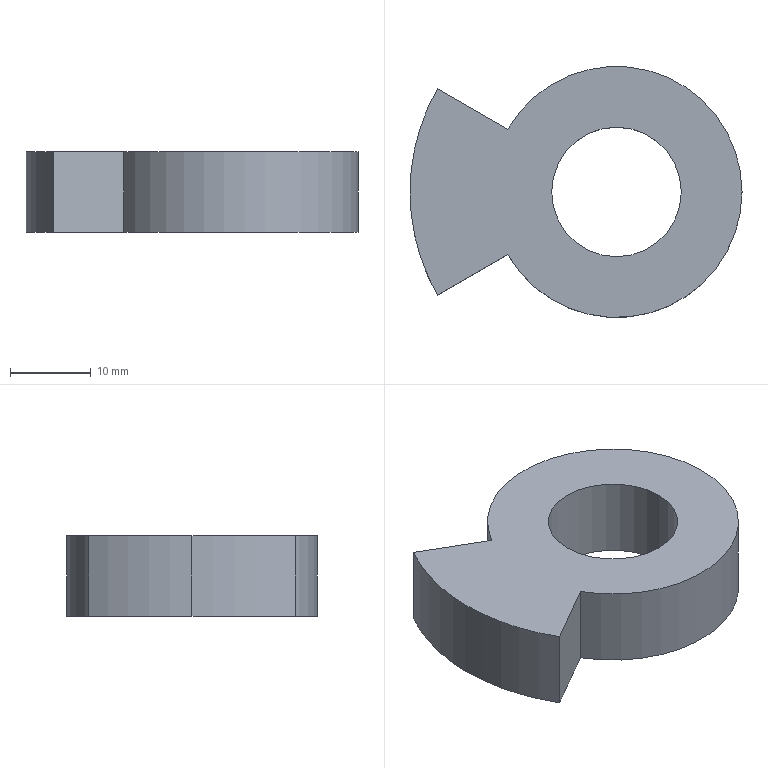Part | STEP file | Sensing plate | 1 solid | 9 faces | box 41 x 31 x 10 mm | volume 7684 mm3 | cylinder 5 | plane 4 | commonest cylinder face diameters 16 x2 51 x2 31 x1
STEP:
#1=CARTESIAN_POINT('',(-8.,0.,5.));
#2=VERTEX_POINT('',#1);
#3=CARTESIAN_POINT('',(8.,0.,5.));
#4=VERTEX_POINT('',#3);
#5=CARTESIAN_POINT('',(0.,0.,5.));
#6=DIRECTION('',(0.,0.,1.));
#7=DIRECTION('',(1.,0.,0.));
#8=AXIS2_PLACEMENT_3D('',#5,#6,#7);
#9=CIRCLE('',#8,8.);
#10=EDGE_CURVE('',#2,#4,#9,.T.);
#11=ORIENTED_EDGE('',*,*,#10,.T.);
#12=CARTESIAN_POINT('',(8.,0.,-5.));
#13=VERTEX_POINT('',#12);
#14=CARTESIAN_POINT('',(8.,0.,5.));
#15=DIRECTION('',(0.,0.,-1.));
#16=VECTOR('',#15,1000.);
#17=LINE('',#14,#16);
#18=EDGE_CURVE('',#4,#13,#17,.T.);
#19=ORIENTED_EDGE('',*,*,#18,.T.);
#20=CARTESIAN_POINT('',(-8.,0.,-5.));
#21=VERTEX_POINT('',#20);
#22=CARTESIAN_POINT('',(0.,0.,-5.));
#23=DIRECTION('',(0.,0.,1.));
#24=DIRECTION('',(1.,0.,0.));
#25=AXIS2_PLACEMENT_3D('',#22,#23,#24);
#26=CIRCLE('',#25,8.);
#27=EDGE_CURVE('',#21,#13,#26,.T.);
#28=ORIENTED_EDGE('',*,*,#27,.F.);
#29=CARTESIAN_POINT('',(-8.,0.,5.));
#30=DIRECTION('',(0.,0.,-1.));
#31=VECTOR('',#30,1000.);
#32=LINE('',#29,#31);
#33=EDGE_CURVE('',#2,#21,#32,.T.);
#34=ORIENTED_EDGE('',*,*,#33,.F.);
#35=EDGE_LOOP('',(#11,#19,#28,#34));
#36=FACE_OUTER_BOUND('',#35,.T.);
#37=CARTESIAN_POINT('',(0.,0.,5.));
#38=DIRECTION('',(0.,0.,-1.));
#39=DIRECTION('',(-1.,0.,0.));
#40=AXIS2_PLACEMENT_3D('',#37,#38,#39);
#41=CYLINDRICAL_SURFACE('',#40,8.);
#42=ADVANCED_FACE('',(#36),#41,.F.);
#43=CARTESIAN_POINT('',(-25.5,0.,5.));
#44=VERTEX_POINT('',#43);
#45=CARTESIAN_POINT('',(-22.084,-12.75,5.));
#46=VERTEX_POINT('',#45);
#47=CARTESIAN_POINT('',(0.,0.,5.));
#48=DIRECTION('',(0.,0.,1.));
#49=DIRECTION('',(1.,0.,0.));
#50=AXIS2_PLACEMENT_3D('',#47,#48,#49);
#51=CIRCLE('',#50,25.5);
#52=EDGE_CURVE('',#44,#46,#51,.T.);
#53=ORIENTED_EDGE('',*,*,#52,.F.);
#54=CARTESIAN_POINT('',(-25.5,0.,-5.));
#55=VERTEX_POINT('',#54);
#56=CARTESIAN_POINT('',(-25.5,0.,5.));
#57=DIRECTION('',(0.,0.,-1.));
#58=VECTOR('',#57,1000.);
#59=LINE('',#56,#58);
#60=EDGE_CURVE('',#44,#55,#59,.T.);
#61=ORIENTED_EDGE('',*,*,#60,.T.);
#62=CARTESIAN_POINT('',(-22.084,-12.75,-5.));
#63=VERTEX_POINT('',#62);
#64=CARTESIAN_POINT('',(0.,0.,-5.));
#65=DIRECTION('',(0.,0.,1.));
#66=DIRECTION('',(1.,0.,0.));
#67=AXIS2_PLACEMENT_3D('',#64,#65,#66);
#68=CIRCLE('',#67,25.5);
#69=EDGE_CURVE('',#55,#63,#68,.T.);
#70=ORIENTED_EDGE('',*,*,#69,.T.);
#71=CARTESIAN_POINT('',(-22.084,-12.75,5.));
#72=DIRECTION('',(0.,0.,-1.));
#73=VECTOR('',#72,1000.);
#74=LINE('',#71,#73);
#75=EDGE_CURVE('',#46,#63,#74,.T.);
#76=ORIENTED_EDGE('',*,*,#75,.F.);
#77=EDGE_LOOP('',(#53,#61,#70,#76));
#78=FACE_OUTER_BOUND('',#77,.T.);
#79=CARTESIAN_POINT('',(0.,0.,5.));
#80=DIRECTION('',(0.,0.,-1.));
#81=DIRECTION('',(-1.,0.,0.));
#82=AXIS2_PLACEMENT_3D('',#79,#80,#81);
#83=CYLINDRICAL_SURFACE('',#82,25.5);
#84=ADVANCED_FACE('',(#78),#83,.T.);
#85=CARTESIAN_POINT('',(-13.423,-7.75,-5.));
#86=VERTEX_POINT('',#85);
#87=CARTESIAN_POINT('',(0.,0.,-5.));
#88=DIRECTION('',(-0.866,-0.5,0.));
#89=VECTOR('',#88,1000.);
#90=LINE('',#87,#89);
#91=EDGE_CURVE('',#86,#63,#90,.T.);
#92=ORIENTED_EDGE('',*,*,#91,.F.);
#93=CARTESIAN_POINT('',(-13.423,-7.75,5.));
#94=VERTEX_POINT('',#93);
#95=CARTESIAN_POINT('',(-13.423,-7.75,5.));
#96=DIRECTION('',(0.,0.,-1.));
#97=VECTOR('',#96,1000.);
#98=LINE('',#95,#97);
#99=EDGE_CURVE('',#94,#86,#98,.T.);
#100=ORIENTED_EDGE('',*,*,#99,.F.);
#101=CARTESIAN_POINT('',(0.,0.,5.));
#102=DIRECTION('',(-0.866,-0.5,0.));
#103=VECTOR('',#102,1000.);
#104=LINE('',#101,#103);
#105=EDGE_CURVE('',#94,#46,#104,.T.);
#106=ORIENTED_EDGE('',*,*,#105,.T.);
#107=ORIENTED_EDGE('',*,*,#75,.T.);
#108=EDGE_LOOP('',(#92,#100,#106,#107));
#109=FACE_OUTER_BOUND('',#108,.T.);
#110=CARTESIAN_POINT('',(0.,0.,5.));
#111=DIRECTION('',(0.5,-0.866,0.));
#112=DIRECTION('',(0.866,0.5,0.));
#113=AXIS2_PLACEMENT_3D('',#110,#111,#112);
#114=PLANE('',#113);
#115=ADVANCED_FACE('',(#109),#114,.T.);
#116=CARTESIAN_POINT('',(-13.423,7.75,-5.));
#117=VERTEX_POINT('',#116);
#118=CARTESIAN_POINT('',(0.,0.,-5.));
#119=DIRECTION('',(0.,0.,1.));
#120=DIRECTION('',(1.,0.,0.));
#121=AXIS2_PLACEMENT_3D('',#118,#119,#120);
#122=CIRCLE('',#121,15.5);
#123=EDGE_CURVE('',#86,#117,#122,.T.);
#124=ORIENTED_EDGE('',*,*,#123,.T.);
#125=CARTESIAN_POINT('',(-13.423,7.75,5.));
#126=VERTEX_POINT('',#125);
#127=CARTESIAN_POINT('',(-13.423,7.75,5.));
#128=DIRECTION('',(0.,0.,-1.));
#129=VECTOR('',#128,1000.);
#130=LINE('',#127,#129);
#131=EDGE_CURVE('',#126,#117,#130,.T.);
#132=ORIENTED_EDGE('',*,*,#131,.F.);
#133=CARTESIAN_POINT('',(0.,0.,5.));
#134=DIRECTION('',(0.,0.,1.));
#135=DIRECTION('',(1.,0.,0.));
#136=AXIS2_PLACEMENT_3D('',#133,#134,#135);
#137=CIRCLE('',#136,15.5);
#138=EDGE_CURVE('',#94,#126,#137,.T.);
#139=ORIENTED_EDGE('',*,*,#138,.F.);
#140=ORIENTED_EDGE('',*,*,#99,.T.);
#141=EDGE_LOOP('',(#124,#132,#139,#140));
#142=FACE_OUTER_BOUND('',#141,.T.);
#143=CARTESIAN_POINT('',(0.,0.,5.));
#144=DIRECTION('',(0.,0.,-1.));
#145=DIRECTION('',(-1.,0.,0.));
#146=AXIS2_PLACEMENT_3D('',#143,#144,#145);
#147=CYLINDRICAL_SURFACE('',#146,15.5);
#148=ADVANCED_FACE('',(#142),#147,.T.);
#149=CARTESIAN_POINT('',(-22.084,12.75,-5.));
#150=VERTEX_POINT('',#149);
#151=CARTESIAN_POINT('',(0.,0.,-5.));
#152=DIRECTION('',(-0.866,0.5,0.));
#153=VECTOR('',#152,1000.);
#154=LINE('',#151,#153);
#155=EDGE_CURVE('',#117,#150,#154,.T.);
#156=ORIENTED_EDGE('',*,*,#155,.T.);
#157=CARTESIAN_POINT('',(-22.084,12.75,5.));
#158=VERTEX_POINT('',#157);
#159=CARTESIAN_POINT('',(-22.084,12.75,5.));
#160=DIRECTION('',(0.,0.,-1.));
#161=VECTOR('',#160,1000.);
#162=LINE('',#159,#161);
#163=EDGE_CURVE('',#158,#150,#162,.T.);
#164=ORIENTED_EDGE('',*,*,#163,.F.);
#165=CARTESIAN_POINT('',(0.,0.,5.));
#166=DIRECTION('',(-0.866,0.5,0.));
#167=VECTOR('',#166,1000.);
#168=LINE('',#165,#167);
#169=EDGE_CURVE('',#126,#158,#168,.T.);
#170=ORIENTED_EDGE('',*,*,#169,.F.);
#171=ORIENTED_EDGE('',*,*,#131,.T.);
#172=EDGE_LOOP('',(#156,#164,#170,#171));
#173=FACE_OUTER_BOUND('',#172,.T.);
#174=CARTESIAN_POINT('',(0.,0.,5.));
#175=DIRECTION('',(-0.5,-0.866,0.));
#176=DIRECTION('',(0.866,-0.5,0.));
#177=AXIS2_PLACEMENT_3D('',#174,#175,#176);
#178=PLANE('',#177);
#179=ADVANCED_FACE('',(#173),#178,.F.);
#180=ORIENTED_EDGE('',*,*,#60,.F.);
#181=CARTESIAN_POINT('',(0.,0.,5.));
#182=DIRECTION('',(0.,0.,1.));
#183=DIRECTION('',(1.,0.,0.));
#184=AXIS2_PLACEMENT_3D('',#181,#182,#183);
#185=CIRCLE('',#184,25.5);
#186=EDGE_CURVE('',#158,#44,#185,.T.);
#187=ORIENTED_EDGE('',*,*,#186,.F.);
#188=ORIENTED_EDGE('',*,*,#163,.T.);
#189=CARTESIAN_POINT('',(0.,0.,-5.));
#190=DIRECTION('',(0.,0.,1.));
#191=DIRECTION('',(1.,0.,0.));
#192=AXIS2_PLACEMENT_3D('',#189,#190,#191);
#193=CIRCLE('',#192,25.5);
#194=EDGE_CURVE('',#150,#55,#193,.T.);
#195=ORIENTED_EDGE('',*,*,#194,.T.);
#196=EDGE_LOOP('',(#180,#187,#188,#195));
#197=FACE_OUTER_BOUND('',#196,.T.);
#198=CARTESIAN_POINT('',(0.,0.,5.));
#199=DIRECTION('',(0.,0.,-1.));
#200=DIRECTION('',(-1.,0.,0.));
#201=AXIS2_PLACEMENT_3D('',#198,#199,#200);
#202=CYLINDRICAL_SURFACE('',#201,25.5);
#203=ADVANCED_FACE('',(#197),#202,.T.);
#204=ORIENTED_EDGE('',*,*,#18,.F.);
#205=CARTESIAN_POINT('',(0.,0.,5.));
#206=DIRECTION('',(0.,0.,1.));
#207=DIRECTION('',(1.,0.,0.));
#208=AXIS2_PLACEMENT_3D('',#205,#206,#207);
#209=CIRCLE('',#208,8.);
#210=EDGE_CURVE('',#4,#2,#209,.T.);
#211=ORIENTED_EDGE('',*,*,#210,.T.);
#212=ORIENTED_EDGE('',*,*,#33,.T.);
#213=CARTESIAN_POINT('',(0.,0.,-5.));
#214=DIRECTION('',(0.,0.,1.));
#215=DIRECTION('',(1.,0.,0.));
#216=AXIS2_PLACEMENT_3D('',#213,#214,#215);
#217=CIRCLE('',#216,8.);
#218=EDGE_CURVE('',#13,#21,#217,.T.);
#219=ORIENTED_EDGE('',*,*,#218,.F.);
#220=EDGE_LOOP('',(#204,#211,#212,#219));
#221=FACE_OUTER_BOUND('',#220,.T.);
#222=CARTESIAN_POINT('',(0.,0.,5.));
#223=DIRECTION('',(0.,0.,-1.));
#224=DIRECTION('',(-1.,0.,0.));
#225=AXIS2_PLACEMENT_3D('',#222,#223,#224);
#226=CYLINDRICAL_SURFACE('',#225,8.);
#227=ADVANCED_FACE('',(#221),#226,.F.);
#228=ORIENTED_EDGE('',*,*,#105,.F.);
#229=ORIENTED_EDGE('',*,*,#138,.T.);
#230=ORIENTED_EDGE('',*,*,#169,.T.);
#231=ORIENTED_EDGE('',*,*,#186,.T.);
#232=ORIENTED_EDGE('',*,*,#52,.T.);
#233=EDGE_LOOP('',(#228,#229,#230,#231,#232));
#234=FACE_OUTER_BOUND('',#233,.T.);
#235=ORIENTED_EDGE('',*,*,#10,.F.);
#236=ORIENTED_EDGE('',*,*,#210,.F.);
#237=EDGE_LOOP('',(#235,#236));
#238=FACE_BOUND('',#237,.T.);
#239=CARTESIAN_POINT('',(0.,0.,5.));
#240=DIRECTION('',(0.,0.,1.));
#241=DIRECTION('',(1.,0.,0.));
#242=AXIS2_PLACEMENT_3D('',#239,#240,#241);
#243=PLANE('',#242);
#244=ADVANCED_FACE('',(#234,#238),#243,.T.);
#245=ORIENTED_EDGE('',*,*,#91,.T.);
#246=ORIENTED_EDGE('',*,*,#69,.F.);
#247=ORIENTED_EDGE('',*,*,#194,.F.);
#248=ORIENTED_EDGE('',*,*,#155,.F.);
#249=ORIENTED_EDGE('',*,*,#123,.F.);
#250=EDGE_LOOP('',(#245,#246,#247,#248,#249));
#251=FACE_OUTER_BOUND('',#250,.T.);
#252=ORIENTED_EDGE('',*,*,#27,.T.);
#253=ORIENTED_EDGE('',*,*,#218,.T.);
#254=EDGE_LOOP('',(#252,#253));
#255=FACE_BOUND('',#254,.T.);
#256=CARTESIAN_POINT('',(0.,0.,-5.));
#257=DIRECTION('',(0.,0.,1.));
#258=DIRECTION('',(1.,0.,0.));
#259=AXIS2_PLACEMENT_3D('',#256,#257,#258);
#260=PLANE('',#259);
#261=ADVANCED_FACE('',(#251,#255),#260,.F.);
#262=CLOSED_SHELL('',(#42,#84,#115,#148,#179,#203,#227,#244,#261));
#263=MANIFOLD_SOLID_BREP('',#262);
#264=CARTESIAN_POINT('',(0.,0.,0.));
#265=DIRECTION('',(0.,0.,1.));
#266=DIRECTION('',(1.,0.,0.));
#267=AXIS2_PLACEMENT_3D('',#264,#265,#266);
#268=(LENGTH_UNIT()NAMED_UNIT(*)SI_UNIT(.MILLI.,.METRE.));
#269=UNCERTAINTY_MEASURE_WITH_UNIT(LENGTH_MEASURE(0.00001),#268,'','');
#270=(NAMED_UNIT(*)PLANE_ANGLE_UNIT()SI_UNIT($,.RADIAN.));
#271=(NAMED_UNIT(*)SI_UNIT($,.STERADIAN.)SOLID_ANGLE_UNIT());
#272=(GEOMETRIC_REPRESENTATION_CONTEXT(3)GLOBAL_UNCERTAINTY_ASSIGNED_CONTEXT((#269))GLOBAL_UNIT_ASSIGNED_CONTEXT((#268,#270,#271))REPRESENTATION_CONTEXT('',''));
#273=ADVANCED_BREP_SHAPE_REPRESENTATION('',(#263,#267),#272);